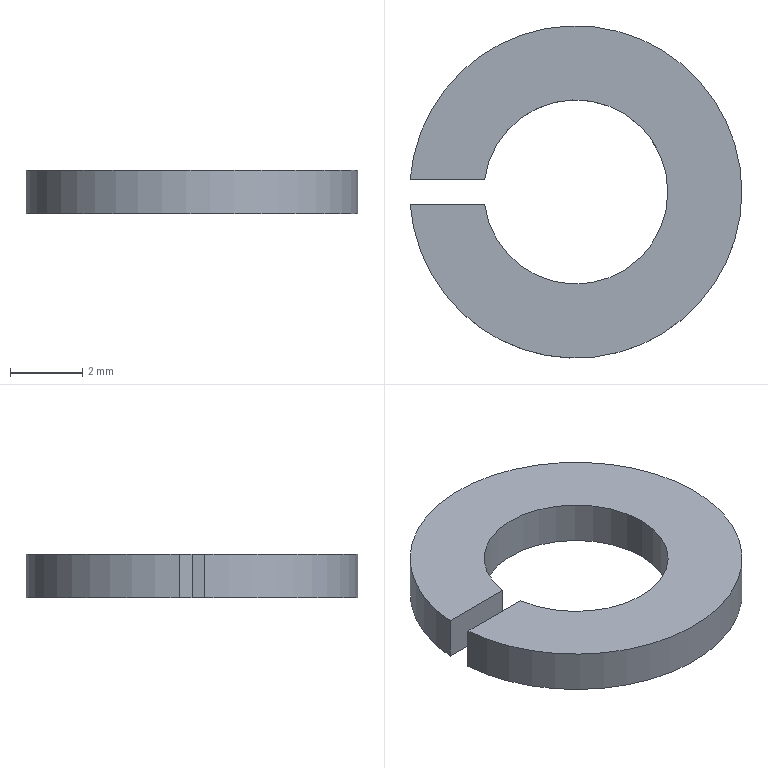Part | SolidWorks | features Extrusion 1 | 1 solid | 8 faces | box 9.187 x 9.2 x 1.2 mm | volume 53.532 mm3 | cylinder 4 | plane 4 | commonest cylinder face diameters 5.1 x2 9.2 x2
STEP:
#1=CARTESIAN_POINT('',(-2.526,0.35,0.));
#2=VERTEX_POINT('',#1);
#3=CARTESIAN_POINT('',(2.55,0.,0.));
#4=VERTEX_POINT('',#3);
#5=CARTESIAN_POINT('',(0.,0.,0.));
#6=DIRECTION('',(0.,0.,-1.));
#7=DIRECTION('',(-1.,0.,0.));
#8=AXIS2_PLACEMENT_3D('',#5,#6,#7);
#9=CIRCLE('',#8,2.55);
#10=EDGE_CURVE('',#2,#4,#9,.T.);
#11=ORIENTED_EDGE('',*,*,#10,.T.);
#12=CARTESIAN_POINT('',(2.55,0.,1.2));
#13=VERTEX_POINT('',#12);
#14=CARTESIAN_POINT('',(2.55,0.,0.));
#15=DIRECTION('',(0.,0.,1.));
#16=VECTOR('',#15,1000.);
#17=LINE('',#14,#16);
#18=EDGE_CURVE('',#4,#13,#17,.T.);
#19=ORIENTED_EDGE('',*,*,#18,.T.);
#20=CARTESIAN_POINT('',(-2.526,0.35,1.2));
#21=VERTEX_POINT('',#20);
#22=CARTESIAN_POINT('',(0.,0.,1.2));
#23=DIRECTION('',(0.,0.,-1.));
#24=DIRECTION('',(-1.,0.,0.));
#25=AXIS2_PLACEMENT_3D('',#22,#23,#24);
#26=CIRCLE('',#25,2.55);
#27=EDGE_CURVE('',#21,#13,#26,.T.);
#28=ORIENTED_EDGE('',*,*,#27,.F.);
#29=CARTESIAN_POINT('',(-2.526,0.35,0.));
#30=DIRECTION('',(0.,0.,1.));
#31=VECTOR('',#30,1000.);
#32=LINE('',#29,#31);
#33=EDGE_CURVE('',#2,#21,#32,.T.);
#34=ORIENTED_EDGE('',*,*,#33,.F.);
#35=EDGE_LOOP('',(#11,#19,#28,#34));
#36=FACE_OUTER_BOUND('',#35,.T.);
#37=CARTESIAN_POINT('',(0.,0.,0.));
#38=DIRECTION('',(0.,0.,1.));
#39=DIRECTION('',(1.,0.,0.));
#40=AXIS2_PLACEMENT_3D('',#37,#38,#39);
#41=CYLINDRICAL_SURFACE('',#40,2.55);
#42=ADVANCED_FACE('',(#36),#41,.F.);
#43=CARTESIAN_POINT('',(-4.587,-0.35,0.));
#44=VERTEX_POINT('',#43);
#45=CARTESIAN_POINT('',(4.6,0.,0.));
#46=VERTEX_POINT('',#45);
#47=CARTESIAN_POINT('',(0.,0.,0.));
#48=DIRECTION('',(0.,0.,1.));
#49=DIRECTION('',(1.,0.,0.));
#50=AXIS2_PLACEMENT_3D('',#47,#48,#49);
#51=CIRCLE('',#50,4.6);
#52=EDGE_CURVE('',#44,#46,#51,.T.);
#53=ORIENTED_EDGE('',*,*,#52,.T.);
#54=CARTESIAN_POINT('',(4.6,0.,1.2));
#55=VERTEX_POINT('',#54);
#56=CARTESIAN_POINT('',(4.6,0.,0.));
#57=DIRECTION('',(0.,0.,1.));
#58=VECTOR('',#57,1000.);
#59=LINE('',#56,#58);
#60=EDGE_CURVE('',#46,#55,#59,.T.);
#61=ORIENTED_EDGE('',*,*,#60,.T.);
#62=CARTESIAN_POINT('',(-4.587,-0.35,1.2));
#63=VERTEX_POINT('',#62);
#64=CARTESIAN_POINT('',(0.,0.,1.2));
#65=DIRECTION('',(0.,0.,1.));
#66=DIRECTION('',(1.,0.,0.));
#67=AXIS2_PLACEMENT_3D('',#64,#65,#66);
#68=CIRCLE('',#67,4.6);
#69=EDGE_CURVE('',#63,#55,#68,.T.);
#70=ORIENTED_EDGE('',*,*,#69,.F.);
#71=CARTESIAN_POINT('',(-4.587,-0.35,0.));
#72=DIRECTION('',(0.,0.,1.));
#73=VECTOR('',#72,1000.);
#74=LINE('',#71,#73);
#75=EDGE_CURVE('',#44,#63,#74,.T.);
#76=ORIENTED_EDGE('',*,*,#75,.F.);
#77=EDGE_LOOP('',(#53,#61,#70,#76));
#78=FACE_OUTER_BOUND('',#77,.T.);
#79=CARTESIAN_POINT('',(0.,0.,0.));
#80=DIRECTION('',(0.,0.,1.));
#81=DIRECTION('',(1.,0.,0.));
#82=AXIS2_PLACEMENT_3D('',#79,#80,#81);
#83=CYLINDRICAL_SURFACE('',#82,4.6);
#84=ADVANCED_FACE('',(#78),#83,.T.);
#85=ORIENTED_EDGE('',*,*,#60,.F.);
#86=CARTESIAN_POINT('',(-4.587,0.35,0.));
#87=VERTEX_POINT('',#86);
#88=CARTESIAN_POINT('',(0.,0.,0.));
#89=DIRECTION('',(0.,0.,1.));
#90=DIRECTION('',(1.,0.,0.));
#91=AXIS2_PLACEMENT_3D('',#88,#89,#90);
#92=CIRCLE('',#91,4.6);
#93=EDGE_CURVE('',#46,#87,#92,.T.);
#94=ORIENTED_EDGE('',*,*,#93,.T.);
#95=CARTESIAN_POINT('',(-4.587,0.35,1.2));
#96=VERTEX_POINT('',#95);
#97=CARTESIAN_POINT('',(-4.587,0.35,0.));
#98=DIRECTION('',(0.,0.,1.));
#99=VECTOR('',#98,1000.);
#100=LINE('',#97,#99);
#101=EDGE_CURVE('',#87,#96,#100,.T.);
#102=ORIENTED_EDGE('',*,*,#101,.T.);
#103=CARTESIAN_POINT('',(0.,0.,1.2));
#104=DIRECTION('',(0.,0.,1.));
#105=DIRECTION('',(1.,0.,0.));
#106=AXIS2_PLACEMENT_3D('',#103,#104,#105);
#107=CIRCLE('',#106,4.6);
#108=EDGE_CURVE('',#55,#96,#107,.T.);
#109=ORIENTED_EDGE('',*,*,#108,.F.);
#110=EDGE_LOOP('',(#85,#94,#102,#109));
#111=FACE_OUTER_BOUND('',#110,.T.);
#112=CARTESIAN_POINT('',(0.,0.,0.));
#113=DIRECTION('',(0.,0.,1.));
#114=DIRECTION('',(1.,0.,0.));
#115=AXIS2_PLACEMENT_3D('',#112,#113,#114);
#116=CYLINDRICAL_SURFACE('',#115,4.6);
#117=ADVANCED_FACE('',(#111),#116,.T.);
#118=CARTESIAN_POINT('',(-2.526,-0.35,1.2));
#119=VERTEX_POINT('',#118);
#120=CARTESIAN_POINT('',(-2.526,-0.35,1.2));
#121=DIRECTION('',(-1.,0.,0.));
#122=VECTOR('',#121,1000.);
#123=LINE('',#120,#122);
#124=EDGE_CURVE('',#119,#63,#123,.T.);
#125=ORIENTED_EDGE('',*,*,#124,.F.);
#126=CARTESIAN_POINT('',(-2.526,-0.35,0.));
#127=VERTEX_POINT('',#126);
#128=CARTESIAN_POINT('',(-2.526,-0.35,0.));
#129=DIRECTION('',(0.,0.,1.));
#130=VECTOR('',#129,1000.);
#131=LINE('',#128,#130);
#132=EDGE_CURVE('',#127,#119,#131,.T.);
#133=ORIENTED_EDGE('',*,*,#132,.F.);
#134=CARTESIAN_POINT('',(-2.526,-0.35,0.));
#135=DIRECTION('',(-1.,0.,0.));
#136=VECTOR('',#135,1000.);
#137=LINE('',#134,#136);
#138=EDGE_CURVE('',#127,#44,#137,.T.);
#139=ORIENTED_EDGE('',*,*,#138,.T.);
#140=ORIENTED_EDGE('',*,*,#75,.T.);
#141=EDGE_LOOP('',(#125,#133,#139,#140));
#142=FACE_OUTER_BOUND('',#141,.T.);
#143=CARTESIAN_POINT('',(-2.526,-0.35,0.));
#144=DIRECTION('',(0.,1.,0.));
#145=DIRECTION('',(0.,0.,1.));
#146=AXIS2_PLACEMENT_3D('',#143,#144,#145);
#147=PLANE('',#146);
#148=ADVANCED_FACE('',(#142),#147,.T.);
#149=ORIENTED_EDGE('',*,*,#18,.F.);
#150=CARTESIAN_POINT('',(0.,0.,0.));
#151=DIRECTION('',(0.,0.,-1.));
#152=DIRECTION('',(-1.,0.,0.));
#153=AXIS2_PLACEMENT_3D('',#150,#151,#152);
#154=CIRCLE('',#153,2.55);
#155=EDGE_CURVE('',#4,#127,#154,.T.);
#156=ORIENTED_EDGE('',*,*,#155,.T.);
#157=ORIENTED_EDGE('',*,*,#132,.T.);
#158=CARTESIAN_POINT('',(0.,0.,1.2));
#159=DIRECTION('',(0.,0.,-1.));
#160=DIRECTION('',(-1.,0.,0.));
#161=AXIS2_PLACEMENT_3D('',#158,#159,#160);
#162=CIRCLE('',#161,2.55);
#163=EDGE_CURVE('',#13,#119,#162,.T.);
#164=ORIENTED_EDGE('',*,*,#163,.F.);
#165=EDGE_LOOP('',(#149,#156,#157,#164));
#166=FACE_OUTER_BOUND('',#165,.T.);
#167=CARTESIAN_POINT('',(0.,0.,0.));
#168=DIRECTION('',(0.,0.,1.));
#169=DIRECTION('',(1.,0.,0.));
#170=AXIS2_PLACEMENT_3D('',#167,#168,#169);
#171=CYLINDRICAL_SURFACE('',#170,2.55);
#172=ADVANCED_FACE('',(#166),#171,.F.);
#173=CARTESIAN_POINT('',(-4.587,0.35,1.2));
#174=DIRECTION('',(1.,0.,0.));
#175=VECTOR('',#174,1000.);
#176=LINE('',#173,#175);
#177=EDGE_CURVE('',#96,#21,#176,.T.);
#178=ORIENTED_EDGE('',*,*,#177,.F.);
#179=ORIENTED_EDGE('',*,*,#101,.F.);
#180=CARTESIAN_POINT('',(-4.587,0.35,0.));
#181=DIRECTION('',(1.,0.,0.));
#182=VECTOR('',#181,1000.);
#183=LINE('',#180,#182);
#184=EDGE_CURVE('',#87,#2,#183,.T.);
#185=ORIENTED_EDGE('',*,*,#184,.T.);
#186=ORIENTED_EDGE('',*,*,#33,.T.);
#187=EDGE_LOOP('',(#178,#179,#185,#186));
#188=FACE_OUTER_BOUND('',#187,.T.);
#189=CARTESIAN_POINT('',(-4.587,0.35,0.));
#190=DIRECTION('',(0.,-1.,0.));
#191=DIRECTION('',(1.,0.,0.));
#192=AXIS2_PLACEMENT_3D('',#189,#190,#191);
#193=PLANE('',#192);
#194=ADVANCED_FACE('',(#188),#193,.T.);
#195=ORIENTED_EDGE('',*,*,#52,.F.);
#196=ORIENTED_EDGE('',*,*,#138,.F.);
#197=ORIENTED_EDGE('',*,*,#155,.F.);
#198=ORIENTED_EDGE('',*,*,#10,.F.);
#199=ORIENTED_EDGE('',*,*,#184,.F.);
#200=ORIENTED_EDGE('',*,*,#93,.F.);
#201=EDGE_LOOP('',(#195,#196,#197,#198,#199,#200));
#202=FACE_OUTER_BOUND('',#201,.T.);
#203=CARTESIAN_POINT('',(0.,0.,0.));
#204=DIRECTION('',(0.,0.,1.));
#205=DIRECTION('',(1.,0.,0.));
#206=AXIS2_PLACEMENT_3D('',#203,#204,#205);
#207=PLANE('',#206);
#208=ADVANCED_FACE('',(#202),#207,.F.);
#209=ORIENTED_EDGE('',*,*,#69,.T.);
#210=ORIENTED_EDGE('',*,*,#108,.T.);
#211=ORIENTED_EDGE('',*,*,#177,.T.);
#212=ORIENTED_EDGE('',*,*,#27,.T.);
#213=ORIENTED_EDGE('',*,*,#163,.T.);
#214=ORIENTED_EDGE('',*,*,#124,.T.);
#215=EDGE_LOOP('',(#209,#210,#211,#212,#213,#214));
#216=FACE_OUTER_BOUND('',#215,.T.);
#217=CARTESIAN_POINT('',(0.,0.,1.2));
#218=DIRECTION('',(0.,0.,1.));
#219=DIRECTION('',(1.,0.,0.));
#220=AXIS2_PLACEMENT_3D('',#217,#218,#219);
#221=PLANE('',#220);
#222=ADVANCED_FACE('',(#216),#221,.T.);
#223=CLOSED_SHELL('',(#42,#84,#117,#148,#172,#194,#208,#222));
#224=MANIFOLD_SOLID_BREP('',#223);
#225=CARTESIAN_POINT('',(0.,0.,0.));
#226=DIRECTION('',(0.,0.,1.));
#227=DIRECTION('',(1.,0.,0.));
#228=AXIS2_PLACEMENT_3D('',#225,#226,#227);
#229=(LENGTH_UNIT()NAMED_UNIT(*)SI_UNIT(.MILLI.,.METRE.));
#230=UNCERTAINTY_MEASURE_WITH_UNIT(LENGTH_MEASURE(0.00001),#229,'','');
#231=(NAMED_UNIT(*)PLANE_ANGLE_UNIT()SI_UNIT($,.RADIAN.));
#232=(NAMED_UNIT(*)SI_UNIT($,.STERADIAN.)SOLID_ANGLE_UNIT());
#233=(GEOMETRIC_REPRESENTATION_CONTEXT(3)GLOBAL_UNCERTAINTY_ASSIGNED_CONTEXT((#230))GLOBAL_UNIT_ASSIGNED_CONTEXT((#229,#231,#232))REPRESENTATION_CONTEXT('',''));
#234=ADVANCED_BREP_SHAPE_REPRESENTATION('',(#224,#228),#233);